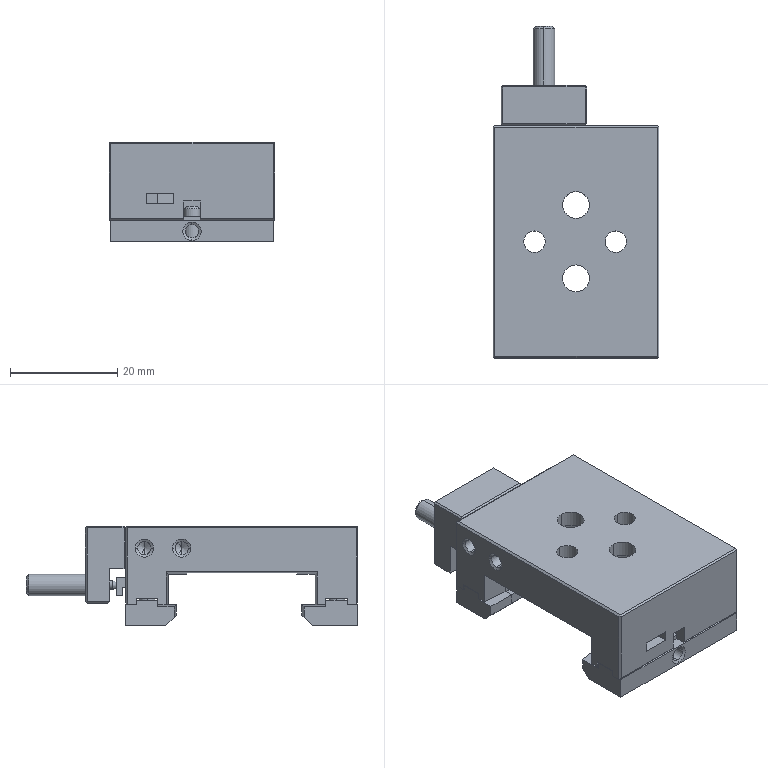Part | NX | 8 solids | 288 faces | box 31 x 62.005 x 18.65 mm | volume 16252 mm3 | plane 144 | cylinder 91 | cone 52 | sphere 1 | commonest cylinder face diameters 2.5 x47 3.3 x10 3 x8 4 x6 3.5 x4 5 x4